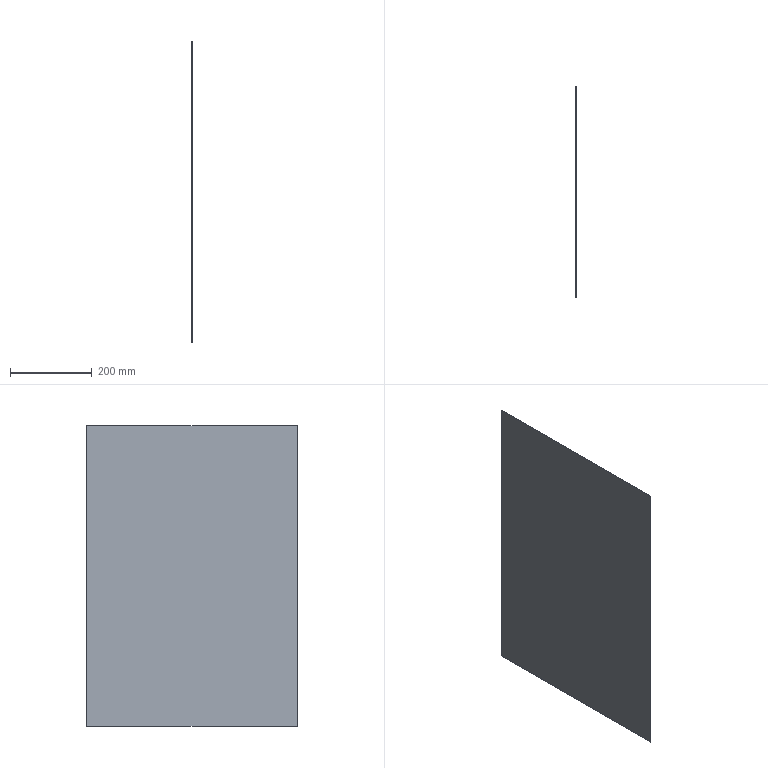Part | SolidWorks | features FlatPattern 1, SMBaseFlange 1, SheetMetal 1 | 1 solid | 6 faces | box 1.2 x 515 x 735 mm | volume 454230 mm3 | plane 6
STEP:
#1=CARTESIAN_POINT('',(20.131,-257.5,-19.791));
#2=VERTEX_POINT('',#1);
#3=CARTESIAN_POINT('',(20.131,-257.5,-754.791));
#4=VERTEX_POINT('',#3);
#5=CARTESIAN_POINT('',(20.131,-257.5,-19.791));
#6=DIRECTION('',(0.,0.,-1.));
#7=VECTOR('',#6,1000.);
#8=LINE('',#5,#7);
#9=EDGE_CURVE('',#2,#4,#8,.T.);
#10=ORIENTED_EDGE('',*,*,#9,.T.);
#11=CARTESIAN_POINT('',(20.131,257.5,-754.791));
#12=VERTEX_POINT('',#11);
#13=CARTESIAN_POINT('',(20.131,257.5,-754.791));
#14=DIRECTION('',(0.,-1.,0.));
#15=VECTOR('',#14,1000.);
#16=LINE('',#13,#15);
#17=EDGE_CURVE('',#12,#4,#16,.T.);
#18=ORIENTED_EDGE('',*,*,#17,.F.);
#19=CARTESIAN_POINT('',(20.131,257.5,-19.791));
#20=VERTEX_POINT('',#19);
#21=CARTESIAN_POINT('',(20.131,257.5,-19.791));
#22=DIRECTION('',(0.,0.,-1.));
#23=VECTOR('',#22,1000.);
#24=LINE('',#21,#23);
#25=EDGE_CURVE('',#20,#12,#24,.T.);
#26=ORIENTED_EDGE('',*,*,#25,.F.);
#27=CARTESIAN_POINT('',(20.131,257.5,-19.791));
#28=DIRECTION('',(0.,-1.,0.));
#29=VECTOR('',#28,1000.);
#30=LINE('',#27,#29);
#31=EDGE_CURVE('',#20,#2,#30,.T.);
#32=ORIENTED_EDGE('',*,*,#31,.T.);
#33=EDGE_LOOP('',(#10,#18,#26,#32));
#34=FACE_OUTER_BOUND('',#33,.T.);
#35=CARTESIAN_POINT('',(20.131,257.5,-19.791));
#36=DIRECTION('',(-1.,0.,0.));
#37=DIRECTION('',(0.,0.,1.));
#38=AXIS2_PLACEMENT_3D('',#35,#36,#37);
#39=PLANE('',#38);
#40=ADVANCED_FACE('',(#34),#39,.F.);
#41=CARTESIAN_POINT('',(18.931,-257.5,-754.791));
#42=VERTEX_POINT('',#41);
#43=CARTESIAN_POINT('',(18.931,-257.5,-754.791));
#44=DIRECTION('',(1.,0.,0.));
#45=VECTOR('',#44,1000.);
#46=LINE('',#43,#45);
#47=EDGE_CURVE('',#42,#4,#46,.T.);
#48=ORIENTED_EDGE('',*,*,#47,.F.);
#49=CARTESIAN_POINT('',(18.931,257.5,-754.791));
#50=VERTEX_POINT('',#49);
#51=CARTESIAN_POINT('',(18.931,257.5,-754.791));
#52=DIRECTION('',(0.,-1.,0.));
#53=VECTOR('',#52,1000.);
#54=LINE('',#51,#53);
#55=EDGE_CURVE('',#50,#42,#54,.T.);
#56=ORIENTED_EDGE('',*,*,#55,.F.);
#57=CARTESIAN_POINT('',(18.931,257.5,-754.791));
#58=DIRECTION('',(1.,0.,0.));
#59=VECTOR('',#58,1000.);
#60=LINE('',#57,#59);
#61=EDGE_CURVE('',#50,#12,#60,.T.);
#62=ORIENTED_EDGE('',*,*,#61,.T.);
#63=ORIENTED_EDGE('',*,*,#17,.T.);
#64=EDGE_LOOP('',(#48,#56,#62,#63));
#65=FACE_OUTER_BOUND('',#64,.T.);
#66=CARTESIAN_POINT('',(18.931,257.5,-754.791));
#67=DIRECTION('',(0.,0.,-1.));
#68=DIRECTION('',(-1.,0.,0.));
#69=AXIS2_PLACEMENT_3D('',#66,#67,#68);
#70=PLANE('',#69);
#71=ADVANCED_FACE('',(#65),#70,.T.);
#72=CARTESIAN_POINT('',(18.931,-257.5,-19.791));
#73=VERTEX_POINT('',#72);
#74=CARTESIAN_POINT('',(18.931,-257.5,-19.791));
#75=DIRECTION('',(0.,0.,-1.));
#76=VECTOR('',#75,1000.);
#77=LINE('',#74,#76);
#78=EDGE_CURVE('',#73,#42,#77,.T.);
#79=ORIENTED_EDGE('',*,*,#78,.F.);
#80=CARTESIAN_POINT('',(18.931,257.5,-19.791));
#81=VERTEX_POINT('',#80);
#82=CARTESIAN_POINT('',(18.931,257.5,-19.791));
#83=DIRECTION('',(0.,-1.,0.));
#84=VECTOR('',#83,1000.);
#85=LINE('',#82,#84);
#86=EDGE_CURVE('',#81,#73,#85,.T.);
#87=ORIENTED_EDGE('',*,*,#86,.F.);
#88=CARTESIAN_POINT('',(18.931,257.5,-19.791));
#89=DIRECTION('',(0.,0.,-1.));
#90=VECTOR('',#89,1000.);
#91=LINE('',#88,#90);
#92=EDGE_CURVE('',#81,#50,#91,.T.);
#93=ORIENTED_EDGE('',*,*,#92,.T.);
#94=ORIENTED_EDGE('',*,*,#55,.T.);
#95=EDGE_LOOP('',(#79,#87,#93,#94));
#96=FACE_OUTER_BOUND('',#95,.T.);
#97=CARTESIAN_POINT('',(18.931,257.5,-19.791));
#98=DIRECTION('',(-1.,0.,0.));
#99=DIRECTION('',(0.,0.,1.));
#100=AXIS2_PLACEMENT_3D('',#97,#98,#99);
#101=PLANE('',#100);
#102=ADVANCED_FACE('',(#96),#101,.T.);
#103=CARTESIAN_POINT('',(20.131,-257.5,-19.791));
#104=DIRECTION('',(-1.,0.,0.));
#105=VECTOR('',#104,1000.);
#106=LINE('',#103,#105);
#107=EDGE_CURVE('',#2,#73,#106,.T.);
#108=ORIENTED_EDGE('',*,*,#107,.F.);
#109=ORIENTED_EDGE('',*,*,#31,.F.);
#110=CARTESIAN_POINT('',(20.131,257.5,-19.791));
#111=DIRECTION('',(-1.,0.,0.));
#112=VECTOR('',#111,1000.);
#113=LINE('',#110,#112);
#114=EDGE_CURVE('',#20,#81,#113,.T.);
#115=ORIENTED_EDGE('',*,*,#114,.T.);
#116=ORIENTED_EDGE('',*,*,#86,.T.);
#117=EDGE_LOOP('',(#108,#109,#115,#116));
#118=FACE_OUTER_BOUND('',#117,.T.);
#119=CARTESIAN_POINT('',(20.131,257.5,-19.791));
#120=DIRECTION('',(0.,0.,1.));
#121=DIRECTION('',(1.,0.,0.));
#122=AXIS2_PLACEMENT_3D('',#119,#120,#121);
#123=PLANE('',#122);
#124=ADVANCED_FACE('',(#118),#123,.T.);
#125=ORIENTED_EDGE('',*,*,#25,.T.);
#126=ORIENTED_EDGE('',*,*,#61,.F.);
#127=ORIENTED_EDGE('',*,*,#92,.F.);
#128=ORIENTED_EDGE('',*,*,#114,.F.);
#129=EDGE_LOOP('',(#125,#126,#127,#128));
#130=FACE_OUTER_BOUND('',#129,.T.);
#131=CARTESIAN_POINT('',(0.,257.5,0.));
#132=DIRECTION('',(0.,-1.,0.));
#133=DIRECTION('',(-1.,0.,0.));
#134=AXIS2_PLACEMENT_3D('',#131,#132,#133);
#135=PLANE('',#134);
#136=ADVANCED_FACE('',(#130),#135,.F.);
#137=ORIENTED_EDGE('',*,*,#9,.F.);
#138=ORIENTED_EDGE('',*,*,#107,.T.);
#139=ORIENTED_EDGE('',*,*,#78,.T.);
#140=ORIENTED_EDGE('',*,*,#47,.T.);
#141=EDGE_LOOP('',(#137,#138,#139,#140));
#142=FACE_OUTER_BOUND('',#141,.T.);
#143=CARTESIAN_POINT('',(0.,-257.5,0.));
#144=DIRECTION('',(0.,-1.,0.));
#145=DIRECTION('',(-1.,0.,0.));
#146=AXIS2_PLACEMENT_3D('',#143,#144,#145);
#147=PLANE('',#146);
#148=ADVANCED_FACE('',(#142),#147,.T.);
#149=CLOSED_SHELL('',(#40,#71,#102,#124,#136,#148));
#150=MANIFOLD_SOLID_BREP('',#149);
#151=CARTESIAN_POINT('',(0.,0.,0.));
#152=DIRECTION('',(0.,0.,1.));
#153=DIRECTION('',(1.,0.,0.));
#154=AXIS2_PLACEMENT_3D('',#151,#152,#153);
#155=(LENGTH_UNIT()NAMED_UNIT(*)SI_UNIT(.MILLI.,.METRE.));
#156=UNCERTAINTY_MEASURE_WITH_UNIT(LENGTH_MEASURE(0.00001),#155,'','');
#157=(NAMED_UNIT(*)PLANE_ANGLE_UNIT()SI_UNIT($,.RADIAN.));
#158=(NAMED_UNIT(*)SI_UNIT($,.STERADIAN.)SOLID_ANGLE_UNIT());
#159=(GEOMETRIC_REPRESENTATION_CONTEXT(3)GLOBAL_UNCERTAINTY_ASSIGNED_CONTEXT((#156))GLOBAL_UNIT_ASSIGNED_CONTEXT((#155,#157,#158))REPRESENTATION_CONTEXT('',''));
#160=ADVANCED_BREP_SHAPE_REPRESENTATION('',(#150,#154),#159);